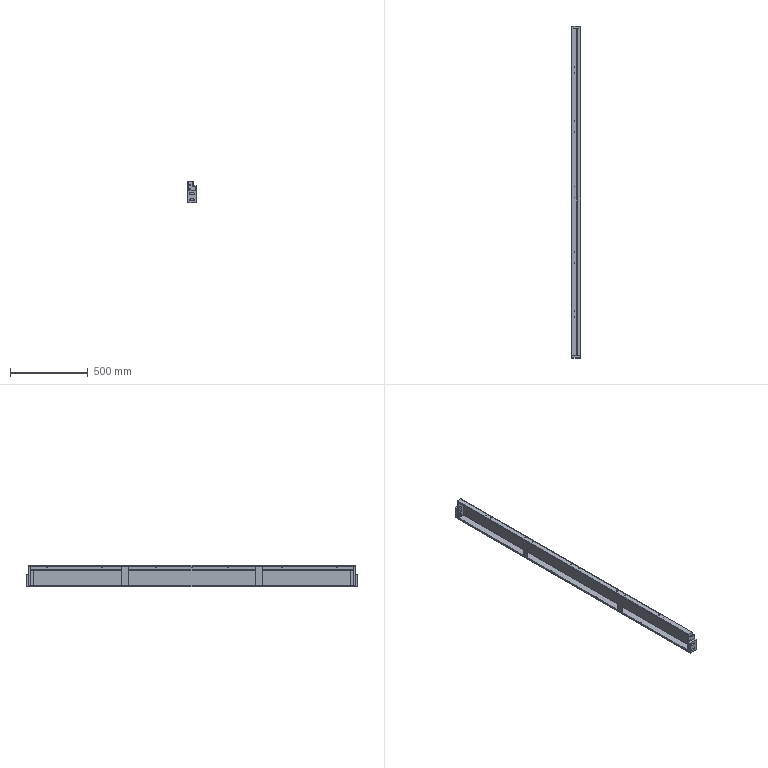Part | SolidWorks | 7 solids | 254 faces | box 58 x 2132 x 140 mm | volume 854542 mm3 | plane 142 | cylinder 112 | commonest cylinder face diameters 5 x32 11 x32 9 x18 4.6 x14 2 x10 4.4 x6